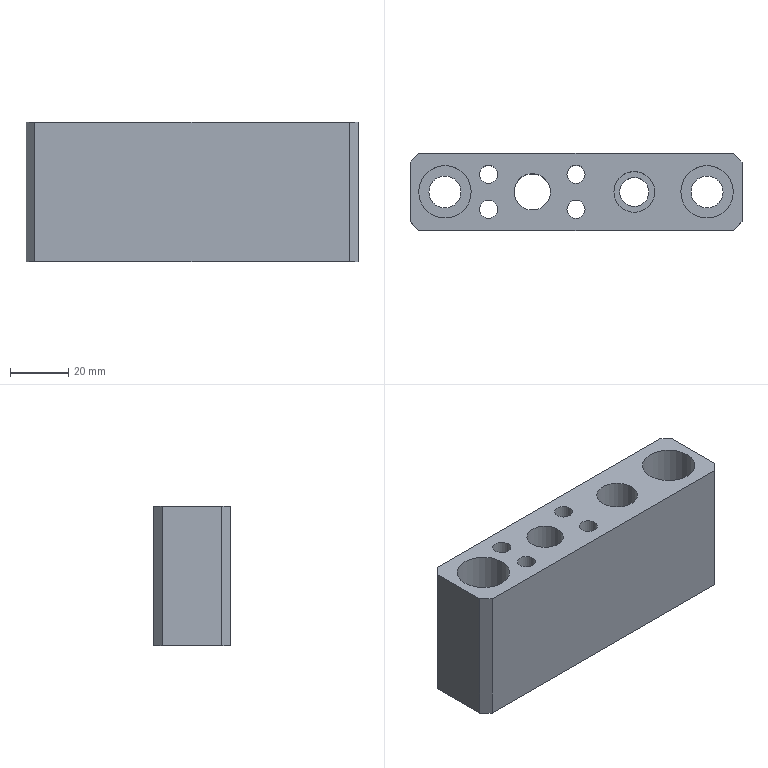Part | STEP file | gslz 2016.10.28-13_id1358_x_t | 1 solid | 32 faces | box 114 x 26.5 x 48 mm | volume 106202 mm3 | plane 17 | cylinder 15 | commonest cylinder face diameters 6.2 x4 8.5 x4 11 x2 18 x2 10 x1 12.5 x1